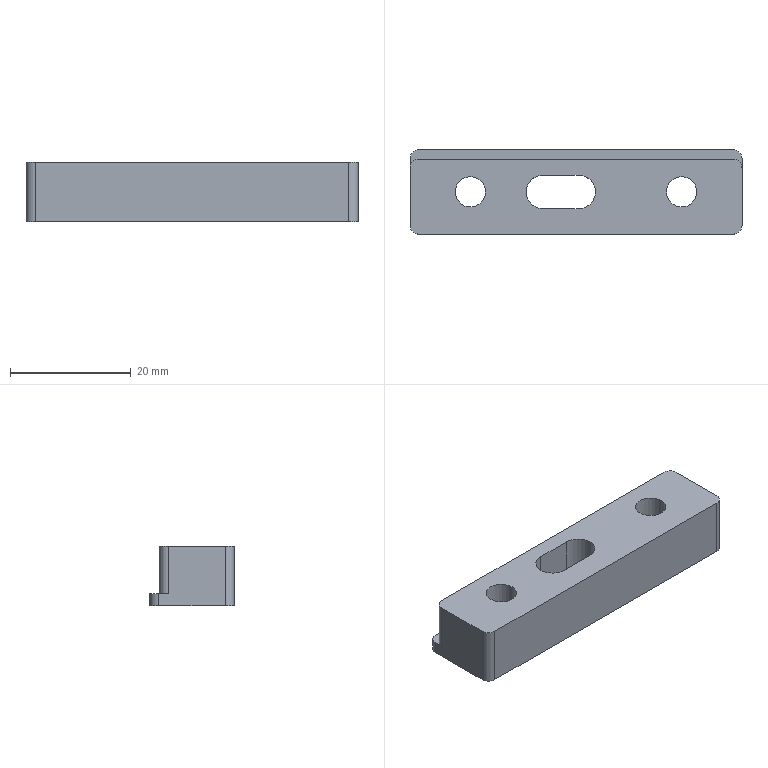Part | STEP file | 1 solid | 20 faces | box 55 x 14 x 9.8 mm | volume 5918 mm3 | plane 10 | cylinder 10 | commonest cylinder face diameters 3 x6 5.02 x2 5.5 x2